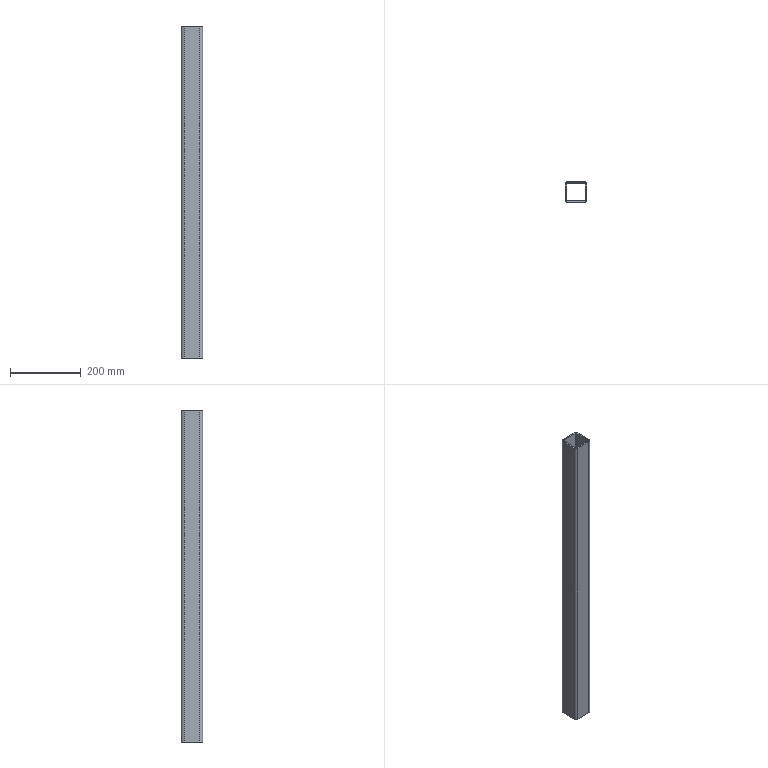Part | SolidWorks | features ICE 1, LibraryFeature 1 | 1 solid | 18 faces | box 60 x 60 x 940 mm | volume 803509 mm3 | plane 10 | cylinder 8 | commonest cylinder face diameters 8 x4 16 x4
STEP:
#1=CARTESIAN_POINT('',(22.,30.,0.));
#2=VERTEX_POINT('',#1);
#3=CARTESIAN_POINT('',(-22.,30.,0.));
#4=VERTEX_POINT('',#3);
#5=CARTESIAN_POINT('',(0.,30.,0.));
#6=DIRECTION('',(-1.,0.,0.));
#7=VECTOR('',#6,1000.);
#8=LINE('',#5,#7);
#9=EDGE_CURVE('',#2,#4,#8,.T.);
#10=ORIENTED_EDGE('',*,*,#9,.T.);
#11=CARTESIAN_POINT('',(-22.,30.,940.));
#12=VERTEX_POINT('',#11);
#13=CARTESIAN_POINT('',(-22.,30.,940.));
#14=DIRECTION('',(0.,0.,-1.));
#15=VECTOR('',#14,1000.);
#16=LINE('',#13,#15);
#17=EDGE_CURVE('',#12,#4,#16,.T.);
#18=ORIENTED_EDGE('',*,*,#17,.F.);
#19=CARTESIAN_POINT('',(22.,30.,940.));
#20=VERTEX_POINT('',#19);
#21=CARTESIAN_POINT('',(0.,30.,940.));
#22=DIRECTION('',(-1.,0.,0.));
#23=VECTOR('',#22,1000.);
#24=LINE('',#21,#23);
#25=EDGE_CURVE('',#20,#12,#24,.T.);
#26=ORIENTED_EDGE('',*,*,#25,.F.);
#27=CARTESIAN_POINT('',(22.,30.,940.));
#28=DIRECTION('',(0.,0.,-1.));
#29=VECTOR('',#28,1000.);
#30=LINE('',#27,#29);
#31=EDGE_CURVE('',#20,#2,#30,.T.);
#32=ORIENTED_EDGE('',*,*,#31,.T.);
#33=EDGE_LOOP('',(#10,#18,#26,#32));
#34=FACE_OUTER_BOUND('',#33,.T.);
#35=CARTESIAN_POINT('',(0.,30.,940.));
#36=DIRECTION('',(0.,-1.,0.));
#37=DIRECTION('',(0.,0.,-1.));
#38=AXIS2_PLACEMENT_3D('',#35,#36,#37);
#39=PLANE('',#38);
#40=ADVANCED_FACE('',(#34),#39,.F.);
#41=CARTESIAN_POINT('',(-30.,22.,0.));
#42=VERTEX_POINT('',#41);
#43=CARTESIAN_POINT('',(-22.,22.,0.));
#44=DIRECTION('',(0.,0.,1.));
#45=DIRECTION('',(1.,0.,0.));
#46=AXIS2_PLACEMENT_3D('',#43,#44,#45);
#47=CIRCLE('',#46,8.);
#48=EDGE_CURVE('',#4,#42,#47,.T.);
#49=ORIENTED_EDGE('',*,*,#48,.T.);
#50=CARTESIAN_POINT('',(-30.,22.,940.));
#51=VERTEX_POINT('',#50);
#52=CARTESIAN_POINT('',(-30.,22.,940.));
#53=DIRECTION('',(0.,0.,-1.));
#54=VECTOR('',#53,1000.);
#55=LINE('',#52,#54);
#56=EDGE_CURVE('',#51,#42,#55,.T.);
#57=ORIENTED_EDGE('',*,*,#56,.F.);
#58=CARTESIAN_POINT('',(-22.,22.,940.));
#59=DIRECTION('',(0.,0.,1.));
#60=DIRECTION('',(1.,0.,0.));
#61=AXIS2_PLACEMENT_3D('',#58,#59,#60);
#62=CIRCLE('',#61,8.);
#63=EDGE_CURVE('',#12,#51,#62,.T.);
#64=ORIENTED_EDGE('',*,*,#63,.F.);
#65=ORIENTED_EDGE('',*,*,#17,.T.);
#66=EDGE_LOOP('',(#49,#57,#64,#65));
#67=FACE_OUTER_BOUND('',#66,.T.);
#68=CARTESIAN_POINT('',(-22.,22.,940.));
#69=DIRECTION('',(0.,0.,-1.));
#70=DIRECTION('',(-1.,0.,0.));
#71=AXIS2_PLACEMENT_3D('',#68,#69,#70);
#72=CYLINDRICAL_SURFACE('',#71,8.);
#73=ADVANCED_FACE('',(#67),#72,.T.);
#74=CARTESIAN_POINT('',(-30.,-22.,0.));
#75=VERTEX_POINT('',#74);
#76=CARTESIAN_POINT('',(-30.,0.,0.));
#77=DIRECTION('',(0.,1.,0.));
#78=VECTOR('',#77,1000.);
#79=LINE('',#76,#78);
#80=EDGE_CURVE('',#75,#42,#79,.T.);
#81=ORIENTED_EDGE('',*,*,#80,.F.);
#82=CARTESIAN_POINT('',(-30.,-22.,940.));
#83=VERTEX_POINT('',#82);
#84=CARTESIAN_POINT('',(-30.,-22.,940.));
#85=DIRECTION('',(0.,0.,-1.));
#86=VECTOR('',#85,1000.);
#87=LINE('',#84,#86);
#88=EDGE_CURVE('',#83,#75,#87,.T.);
#89=ORIENTED_EDGE('',*,*,#88,.F.);
#90=CARTESIAN_POINT('',(-30.,0.,940.));
#91=DIRECTION('',(0.,1.,0.));
#92=VECTOR('',#91,1000.);
#93=LINE('',#90,#92);
#94=EDGE_CURVE('',#83,#51,#93,.T.);
#95=ORIENTED_EDGE('',*,*,#94,.T.);
#96=ORIENTED_EDGE('',*,*,#56,.T.);
#97=EDGE_LOOP('',(#81,#89,#95,#96));
#98=FACE_OUTER_BOUND('',#97,.T.);
#99=CARTESIAN_POINT('',(-30.,0.,940.));
#100=DIRECTION('',(-1.,0.,0.));
#101=DIRECTION('',(0.,0.,1.));
#102=AXIS2_PLACEMENT_3D('',#99,#100,#101);
#103=PLANE('',#102);
#104=ADVANCED_FACE('',(#98),#103,.T.);
#105=CARTESIAN_POINT('',(-22.,-30.,0.));
#106=VERTEX_POINT('',#105);
#107=CARTESIAN_POINT('',(-22.,-22.,0.));
#108=DIRECTION('',(0.,0.,1.));
#109=DIRECTION('',(1.,0.,0.));
#110=AXIS2_PLACEMENT_3D('',#107,#108,#109);
#111=CIRCLE('',#110,8.);
#112=EDGE_CURVE('',#75,#106,#111,.T.);
#113=ORIENTED_EDGE('',*,*,#112,.T.);
#114=CARTESIAN_POINT('',(-22.,-30.,940.));
#115=VERTEX_POINT('',#114);
#116=CARTESIAN_POINT('',(-22.,-30.,940.));
#117=DIRECTION('',(0.,0.,-1.));
#118=VECTOR('',#117,1000.);
#119=LINE('',#116,#118);
#120=EDGE_CURVE('',#115,#106,#119,.T.);
#121=ORIENTED_EDGE('',*,*,#120,.F.);
#122=CARTESIAN_POINT('',(-22.,-22.,940.));
#123=DIRECTION('',(0.,0.,1.));
#124=DIRECTION('',(1.,0.,0.));
#125=AXIS2_PLACEMENT_3D('',#122,#123,#124);
#126=CIRCLE('',#125,8.);
#127=EDGE_CURVE('',#83,#115,#126,.T.);
#128=ORIENTED_EDGE('',*,*,#127,.F.);
#129=ORIENTED_EDGE('',*,*,#88,.T.);
#130=EDGE_LOOP('',(#113,#121,#128,#129));
#131=FACE_OUTER_BOUND('',#130,.T.);
#132=CARTESIAN_POINT('',(-22.,-22.,940.));
#133=DIRECTION('',(0.,0.,-1.));
#134=DIRECTION('',(-1.,0.,0.));
#135=AXIS2_PLACEMENT_3D('',#132,#133,#134);
#136=CYLINDRICAL_SURFACE('',#135,8.);
#137=ADVANCED_FACE('',(#131),#136,.T.);
#138=CARTESIAN_POINT('',(22.,-30.,0.));
#139=VERTEX_POINT('',#138);
#140=CARTESIAN_POINT('',(0.,-30.,0.));
#141=DIRECTION('',(1.,0.,0.));
#142=VECTOR('',#141,1000.);
#143=LINE('',#140,#142);
#144=EDGE_CURVE('',#106,#139,#143,.T.);
#145=ORIENTED_EDGE('',*,*,#144,.T.);
#146=CARTESIAN_POINT('',(22.,-30.,940.));
#147=VERTEX_POINT('',#146);
#148=CARTESIAN_POINT('',(22.,-30.,940.));
#149=DIRECTION('',(0.,0.,-1.));
#150=VECTOR('',#149,1000.);
#151=LINE('',#148,#150);
#152=EDGE_CURVE('',#147,#139,#151,.T.);
#153=ORIENTED_EDGE('',*,*,#152,.F.);
#154=CARTESIAN_POINT('',(0.,-30.,940.));
#155=DIRECTION('',(1.,0.,0.));
#156=VECTOR('',#155,1000.);
#157=LINE('',#154,#156);
#158=EDGE_CURVE('',#115,#147,#157,.T.);
#159=ORIENTED_EDGE('',*,*,#158,.F.);
#160=ORIENTED_EDGE('',*,*,#120,.T.);
#161=EDGE_LOOP('',(#145,#153,#159,#160));
#162=FACE_OUTER_BOUND('',#161,.T.);
#163=CARTESIAN_POINT('',(0.,-30.,940.));
#164=DIRECTION('',(0.,1.,0.));
#165=DIRECTION('',(0.,0.,1.));
#166=AXIS2_PLACEMENT_3D('',#163,#164,#165);
#167=PLANE('',#166);
#168=ADVANCED_FACE('',(#162),#167,.F.);
#169=CARTESIAN_POINT('',(30.,-22.,0.));
#170=VERTEX_POINT('',#169);
#171=CARTESIAN_POINT('',(22.,-22.,0.));
#172=DIRECTION('',(0.,0.,1.));
#173=DIRECTION('',(1.,0.,0.));
#174=AXIS2_PLACEMENT_3D('',#171,#172,#173);
#175=CIRCLE('',#174,8.);
#176=EDGE_CURVE('',#139,#170,#175,.T.);
#177=ORIENTED_EDGE('',*,*,#176,.T.);
#178=CARTESIAN_POINT('',(30.,-22.,940.));
#179=VERTEX_POINT('',#178);
#180=CARTESIAN_POINT('',(30.,-22.,940.));
#181=DIRECTION('',(0.,0.,-1.));
#182=VECTOR('',#181,1000.);
#183=LINE('',#180,#182);
#184=EDGE_CURVE('',#179,#170,#183,.T.);
#185=ORIENTED_EDGE('',*,*,#184,.F.);
#186=CARTESIAN_POINT('',(22.,-22.,940.));
#187=DIRECTION('',(0.,0.,1.));
#188=DIRECTION('',(1.,0.,0.));
#189=AXIS2_PLACEMENT_3D('',#186,#187,#188);
#190=CIRCLE('',#189,8.);
#191=EDGE_CURVE('',#147,#179,#190,.T.);
#192=ORIENTED_EDGE('',*,*,#191,.F.);
#193=ORIENTED_EDGE('',*,*,#152,.T.);
#194=EDGE_LOOP('',(#177,#185,#192,#193));
#195=FACE_OUTER_BOUND('',#194,.T.);
#196=CARTESIAN_POINT('',(22.,-22.,940.));
#197=DIRECTION('',(0.,0.,-1.));
#198=DIRECTION('',(-1.,0.,0.));
#199=AXIS2_PLACEMENT_3D('',#196,#197,#198);
#200=CYLINDRICAL_SURFACE('',#199,8.);
#201=ADVANCED_FACE('',(#195),#200,.T.);
#202=CARTESIAN_POINT('',(30.,22.,0.));
#203=VERTEX_POINT('',#202);
#204=CARTESIAN_POINT('',(30.,0.,0.));
#205=DIRECTION('',(0.,-1.,0.));
#206=VECTOR('',#205,1000.);
#207=LINE('',#204,#206);
#208=EDGE_CURVE('',#203,#170,#207,.T.);
#209=ORIENTED_EDGE('',*,*,#208,.F.);
#210=CARTESIAN_POINT('',(30.,22.,940.));
#211=VERTEX_POINT('',#210);
#212=CARTESIAN_POINT('',(30.,22.,940.));
#213=DIRECTION('',(0.,0.,-1.));
#214=VECTOR('',#213,1000.);
#215=LINE('',#212,#214);
#216=EDGE_CURVE('',#211,#203,#215,.T.);
#217=ORIENTED_EDGE('',*,*,#216,.F.);
#218=CARTESIAN_POINT('',(30.,0.,940.));
#219=DIRECTION('',(0.,-1.,0.));
#220=VECTOR('',#219,1000.);
#221=LINE('',#218,#220);
#222=EDGE_CURVE('',#211,#179,#221,.T.);
#223=ORIENTED_EDGE('',*,*,#222,.T.);
#224=ORIENTED_EDGE('',*,*,#184,.T.);
#225=EDGE_LOOP('',(#209,#217,#223,#224));
#226=FACE_OUTER_BOUND('',#225,.T.);
#227=CARTESIAN_POINT('',(30.,0.,940.));
#228=DIRECTION('',(1.,0.,0.));
#229=DIRECTION('',(0.,0.,-1.));
#230=AXIS2_PLACEMENT_3D('',#227,#228,#229);
#231=PLANE('',#230);
#232=ADVANCED_FACE('',(#226),#231,.T.);
#233=CARTESIAN_POINT('',(-26.,-22.,0.));
#234=VERTEX_POINT('',#233);
#235=CARTESIAN_POINT('',(-22.,-26.,0.));
#236=VERTEX_POINT('',#235);
#237=CARTESIAN_POINT('',(-22.,-22.,0.));
#238=DIRECTION('',(0.,0.,1.));
#239=DIRECTION('',(1.,0.,0.));
#240=AXIS2_PLACEMENT_3D('',#237,#238,#239);
#241=CIRCLE('',#240,4.);
#242=EDGE_CURVE('',#234,#236,#241,.T.);
#243=ORIENTED_EDGE('',*,*,#242,.F.);
#244=CARTESIAN_POINT('',(-26.,-22.,940.));
#245=VERTEX_POINT('',#244);
#246=CARTESIAN_POINT('',(-26.,-22.,940.));
#247=DIRECTION('',(0.,0.,-1.));
#248=VECTOR('',#247,1000.);
#249=LINE('',#246,#248);
#250=EDGE_CURVE('',#245,#234,#249,.T.);
#251=ORIENTED_EDGE('',*,*,#250,.F.);
#252=CARTESIAN_POINT('',(-22.,-26.,940.));
#253=VERTEX_POINT('',#252);
#254=CARTESIAN_POINT('',(-22.,-22.,940.));
#255=DIRECTION('',(0.,0.,1.));
#256=DIRECTION('',(1.,0.,0.));
#257=AXIS2_PLACEMENT_3D('',#254,#255,#256);
#258=CIRCLE('',#257,4.);
#259=EDGE_CURVE('',#245,#253,#258,.T.);
#260=ORIENTED_EDGE('',*,*,#259,.T.);
#261=CARTESIAN_POINT('',(-22.,-26.,940.));
#262=DIRECTION('',(0.,0.,-1.));
#263=VECTOR('',#262,1000.);
#264=LINE('',#261,#263);
#265=EDGE_CURVE('',#253,#236,#264,.T.);
#266=ORIENTED_EDGE('',*,*,#265,.T.);
#267=EDGE_LOOP('',(#243,#251,#260,#266));
#268=FACE_OUTER_BOUND('',#267,.T.);
#269=CARTESIAN_POINT('',(-22.,-22.,940.));
#270=DIRECTION('',(0.,0.,-1.));
#271=DIRECTION('',(-1.,0.,0.));
#272=AXIS2_PLACEMENT_3D('',#269,#270,#271);
#273=CYLINDRICAL_SURFACE('',#272,4.);
#274=ADVANCED_FACE('',(#268),#273,.F.);
#275=CARTESIAN_POINT('',(-26.,22.,0.));
#276=VERTEX_POINT('',#275);
#277=CARTESIAN_POINT('',(-26.,0.,0.));
#278=DIRECTION('',(0.,1.,0.));
#279=VECTOR('',#278,1000.);
#280=LINE('',#277,#279);
#281=EDGE_CURVE('',#234,#276,#280,.T.);
#282=ORIENTED_EDGE('',*,*,#281,.T.);
#283=CARTESIAN_POINT('',(-26.,22.,940.));
#284=VERTEX_POINT('',#283);
#285=CARTESIAN_POINT('',(-26.,22.,940.));
#286=DIRECTION('',(0.,0.,-1.));
#287=VECTOR('',#286,1000.);
#288=LINE('',#285,#287);
#289=EDGE_CURVE('',#284,#276,#288,.T.);
#290=ORIENTED_EDGE('',*,*,#289,.F.);
#291=CARTESIAN_POINT('',(-26.,0.,940.));
#292=DIRECTION('',(0.,1.,0.));
#293=VECTOR('',#292,1000.);
#294=LINE('',#291,#293);
#295=EDGE_CURVE('',#245,#284,#294,.T.);
#296=ORIENTED_EDGE('',*,*,#295,.F.);
#297=ORIENTED_EDGE('',*,*,#250,.T.);
#298=EDGE_LOOP('',(#282,#290,#296,#297));
#299=FACE_OUTER_BOUND('',#298,.T.);
#300=CARTESIAN_POINT('',(-26.,0.,940.));
#301=DIRECTION('',(-1.,0.,0.));
#302=DIRECTION('',(0.,0.,1.));
#303=AXIS2_PLACEMENT_3D('',#300,#301,#302);
#304=PLANE('',#303);
#305=ADVANCED_FACE('',(#299),#304,.F.);
#306=CARTESIAN_POINT('',(-22.,26.,0.));
#307=VERTEX_POINT('',#306);
#308=CARTESIAN_POINT('',(-22.,22.,0.));
#309=DIRECTION('',(0.,0.,1.));
#310=DIRECTION('',(1.,0.,0.));
#311=AXIS2_PLACEMENT_3D('',#308,#309,#310);
#312=CIRCLE('',#311,4.);
#313=EDGE_CURVE('',#307,#276,#312,.T.);
#314=ORIENTED_EDGE('',*,*,#313,.F.);
#315=CARTESIAN_POINT('',(-22.,26.,940.));
#316=VERTEX_POINT('',#315);
#317=CARTESIAN_POINT('',(-22.,26.,940.));
#318=DIRECTION('',(0.,0.,-1.));
#319=VECTOR('',#318,1000.);
#320=LINE('',#317,#319);
#321=EDGE_CURVE('',#316,#307,#320,.T.);
#322=ORIENTED_EDGE('',*,*,#321,.F.);
#323=CARTESIAN_POINT('',(-22.,22.,940.));
#324=DIRECTION('',(0.,0.,1.));
#325=DIRECTION('',(1.,0.,0.));
#326=AXIS2_PLACEMENT_3D('',#323,#324,#325);
#327=CIRCLE('',#326,4.);
#328=EDGE_CURVE('',#316,#284,#327,.T.);
#329=ORIENTED_EDGE('',*,*,#328,.T.);
#330=ORIENTED_EDGE('',*,*,#289,.T.);
#331=EDGE_LOOP('',(#314,#322,#329,#330));
#332=FACE_OUTER_BOUND('',#331,.T.);
#333=CARTESIAN_POINT('',(-22.,22.,940.));
#334=DIRECTION('',(0.,0.,-1.));
#335=DIRECTION('',(-1.,0.,0.));
#336=AXIS2_PLACEMENT_3D('',#333,#334,#335);
#337=CYLINDRICAL_SURFACE('',#336,4.);
#338=ADVANCED_FACE('',(#332),#337,.F.);
#339=CARTESIAN_POINT('',(22.,26.,0.));
#340=VERTEX_POINT('',#339);
#341=CARTESIAN_POINT('',(0.,26.,0.));
#342=DIRECTION('',(-1.,0.,0.));
#343=VECTOR('',#342,1000.);
#344=LINE('',#341,#343);
#345=EDGE_CURVE('',#340,#307,#344,.T.);
#346=ORIENTED_EDGE('',*,*,#345,.F.);
#347=CARTESIAN_POINT('',(22.,26.,940.));
#348=VERTEX_POINT('',#347);
#349=CARTESIAN_POINT('',(22.,26.,940.));
#350=DIRECTION('',(0.,0.,-1.));
#351=VECTOR('',#350,1000.);
#352=LINE('',#349,#351);
#353=EDGE_CURVE('',#348,#340,#352,.T.);
#354=ORIENTED_EDGE('',*,*,#353,.F.);
#355=CARTESIAN_POINT('',(0.,26.,940.));
#356=DIRECTION('',(-1.,0.,0.));
#357=VECTOR('',#356,1000.);
#358=LINE('',#355,#357);
#359=EDGE_CURVE('',#348,#316,#358,.T.);
#360=ORIENTED_EDGE('',*,*,#359,.T.);
#361=ORIENTED_EDGE('',*,*,#321,.T.);
#362=EDGE_LOOP('',(#346,#354,#360,#361));
#363=FACE_OUTER_BOUND('',#362,.T.);
#364=CARTESIAN_POINT('',(0.,26.,940.));
#365=DIRECTION('',(0.,-1.,0.));
#366=DIRECTION('',(0.,0.,-1.));
#367=AXIS2_PLACEMENT_3D('',#364,#365,#366);
#368=PLANE('',#367);
#369=ADVANCED_FACE('',(#363),#368,.T.);
#370=CARTESIAN_POINT('',(26.,22.,0.));
#371=VERTEX_POINT('',#370);
#372=CARTESIAN_POINT('',(22.,22.,0.));
#373=DIRECTION('',(0.,0.,1.));
#374=DIRECTION('',(1.,0.,0.));
#375=AXIS2_PLACEMENT_3D('',#372,#373,#374);
#376=CIRCLE('',#375,4.);
#377=EDGE_CURVE('',#371,#340,#376,.T.);
#378=ORIENTED_EDGE('',*,*,#377,.F.);
#379=CARTESIAN_POINT('',(26.,22.,940.));
#380=VERTEX_POINT('',#379);
#381=CARTESIAN_POINT('',(26.,22.,940.));
#382=DIRECTION('',(0.,0.,-1.));
#383=VECTOR('',#382,1000.);
#384=LINE('',#381,#383);
#385=EDGE_CURVE('',#380,#371,#384,.T.);
#386=ORIENTED_EDGE('',*,*,#385,.F.);
#387=CARTESIAN_POINT('',(22.,22.,940.));
#388=DIRECTION('',(0.,0.,1.));
#389=DIRECTION('',(1.,0.,0.));
#390=AXIS2_PLACEMENT_3D('',#387,#388,#389);
#391=CIRCLE('',#390,4.);
#392=EDGE_CURVE('',#380,#348,#391,.T.);
#393=ORIENTED_EDGE('',*,*,#392,.T.);
#394=ORIENTED_EDGE('',*,*,#353,.T.);
#395=EDGE_LOOP('',(#378,#386,#393,#394));
#396=FACE_OUTER_BOUND('',#395,.T.);
#397=CARTESIAN_POINT('',(22.,22.,940.));
#398=DIRECTION('',(0.,0.,-1.));
#399=DIRECTION('',(-1.,0.,0.));
#400=AXIS2_PLACEMENT_3D('',#397,#398,#399);
#401=CYLINDRICAL_SURFACE('',#400,4.);
#402=ADVANCED_FACE('',(#396),#401,.F.);
#403=CARTESIAN_POINT('',(26.,-22.,0.));
#404=VERTEX_POINT('',#403);
#405=CARTESIAN_POINT('',(26.,0.,0.));
#406=DIRECTION('',(0.,-1.,0.));
#407=VECTOR('',#406,1000.);
#408=LINE('',#405,#407);
#409=EDGE_CURVE('',#371,#404,#408,.T.);
#410=ORIENTED_EDGE('',*,*,#409,.T.);
#411=CARTESIAN_POINT('',(26.,-22.,940.));
#412=VERTEX_POINT('',#411);
#413=CARTESIAN_POINT('',(26.,-22.,940.));
#414=DIRECTION('',(0.,0.,-1.));
#415=VECTOR('',#414,1000.);
#416=LINE('',#413,#415);
#417=EDGE_CURVE('',#412,#404,#416,.T.);
#418=ORIENTED_EDGE('',*,*,#417,.F.);
#419=CARTESIAN_POINT('',(26.,0.,940.));
#420=DIRECTION('',(0.,-1.,0.));
#421=VECTOR('',#420,1000.);
#422=LINE('',#419,#421);
#423=EDGE_CURVE('',#380,#412,#422,.T.);
#424=ORIENTED_EDGE('',*,*,#423,.F.);
#425=ORIENTED_EDGE('',*,*,#385,.T.);
#426=EDGE_LOOP('',(#410,#418,#424,#425));
#427=FACE_OUTER_BOUND('',#426,.T.);
#428=CARTESIAN_POINT('',(26.,0.,940.));
#429=DIRECTION('',(1.,0.,0.));
#430=DIRECTION('',(0.,0.,-1.));
#431=AXIS2_PLACEMENT_3D('',#428,#429,#430);
#432=PLANE('',#431);
#433=ADVANCED_FACE('',(#427),#432,.F.);
#434=CARTESIAN_POINT('',(22.,-26.,0.));
#435=VERTEX_POINT('',#434);
#436=CARTESIAN_POINT('',(22.,-22.,0.));
#437=DIRECTION('',(0.,0.,1.));
#438=DIRECTION('',(1.,0.,0.));
#439=AXIS2_PLACEMENT_3D('',#436,#437,#438);
#440=CIRCLE('',#439,4.);
#441=EDGE_CURVE('',#435,#404,#440,.T.);
#442=ORIENTED_EDGE('',*,*,#441,.F.);
#443=CARTESIAN_POINT('',(22.,-26.,940.));
#444=VERTEX_POINT('',#443);
#445=CARTESIAN_POINT('',(22.,-26.,940.));
#446=DIRECTION('',(0.,0.,-1.));
#447=VECTOR('',#446,1000.);
#448=LINE('',#445,#447);
#449=EDGE_CURVE('',#444,#435,#448,.T.);
#450=ORIENTED_EDGE('',*,*,#449,.F.);
#451=CARTESIAN_POINT('',(22.,-22.,940.));
#452=DIRECTION('',(0.,0.,1.));
#453=DIRECTION('',(1.,0.,0.));
#454=AXIS2_PLACEMENT_3D('',#451,#452,#453);
#455=CIRCLE('',#454,4.);
#456=EDGE_CURVE('',#444,#412,#455,.T.);
#457=ORIENTED_EDGE('',*,*,#456,.T.);
#458=ORIENTED_EDGE('',*,*,#417,.T.);
#459=EDGE_LOOP('',(#442,#450,#457,#458));
#460=FACE_OUTER_BOUND('',#459,.T.);
#461=CARTESIAN_POINT('',(22.,-22.,940.));
#462=DIRECTION('',(0.,0.,-1.));
#463=DIRECTION('',(-1.,0.,0.));
#464=AXIS2_PLACEMENT_3D('',#461,#462,#463);
#465=CYLINDRICAL_SURFACE('',#464,4.);
#466=ADVANCED_FACE('',(#460),#465,.F.);
#467=CARTESIAN_POINT('',(0.,-26.,0.));
#468=DIRECTION('',(1.,0.,0.));
#469=VECTOR('',#468,1000.);
#470=LINE('',#467,#469);
#471=EDGE_CURVE('',#236,#435,#470,.T.);
#472=ORIENTED_EDGE('',*,*,#471,.F.);
#473=ORIENTED_EDGE('',*,*,#265,.F.);
#474=CARTESIAN_POINT('',(0.,-26.,940.));
#475=DIRECTION('',(1.,0.,0.));
#476=VECTOR('',#475,1000.);
#477=LINE('',#474,#476);
#478=EDGE_CURVE('',#253,#444,#477,.T.);
#479=ORIENTED_EDGE('',*,*,#478,.T.);
#480=ORIENTED_EDGE('',*,*,#449,.T.);
#481=EDGE_LOOP('',(#472,#473,#479,#480));
#482=FACE_OUTER_BOUND('',#481,.T.);
#483=CARTESIAN_POINT('',(0.,-26.,940.));
#484=DIRECTION('',(0.,1.,0.));
#485=DIRECTION('',(0.,0.,1.));
#486=AXIS2_PLACEMENT_3D('',#483,#484,#485);
#487=PLANE('',#486);
#488=ADVANCED_FACE('',(#482),#487,.T.);
#489=CARTESIAN_POINT('',(22.,22.,0.));
#490=DIRECTION('',(0.,0.,1.));
#491=DIRECTION('',(1.,0.,0.));
#492=AXIS2_PLACEMENT_3D('',#489,#490,#491);
#493=CIRCLE('',#492,8.);
#494=EDGE_CURVE('',#203,#2,#493,.T.);
#495=ORIENTED_EDGE('',*,*,#494,.T.);
#496=ORIENTED_EDGE('',*,*,#31,.F.);
#497=CARTESIAN_POINT('',(22.,22.,940.));
#498=DIRECTION('',(0.,0.,1.));
#499=DIRECTION('',(1.,0.,0.));
#500=AXIS2_PLACEMENT_3D('',#497,#498,#499);
#501=CIRCLE('',#500,8.);
#502=EDGE_CURVE('',#211,#20,#501,.T.);
#503=ORIENTED_EDGE('',*,*,#502,.F.);
#504=ORIENTED_EDGE('',*,*,#216,.T.);
#505=EDGE_LOOP('',(#495,#496,#503,#504));
#506=FACE_OUTER_BOUND('',#505,.T.);
#507=CARTESIAN_POINT('',(22.,22.,940.));
#508=DIRECTION('',(0.,0.,-1.));
#509=DIRECTION('',(-1.,0.,0.));
#510=AXIS2_PLACEMENT_3D('',#507,#508,#509);
#511=CYLINDRICAL_SURFACE('',#510,8.);
#512=ADVANCED_FACE('',(#506),#511,.T.);
#513=ORIENTED_EDGE('',*,*,#259,.F.);
#514=ORIENTED_EDGE('',*,*,#295,.T.);
#515=ORIENTED_EDGE('',*,*,#328,.F.);
#516=ORIENTED_EDGE('',*,*,#359,.F.);
#517=ORIENTED_EDGE('',*,*,#392,.F.);
#518=ORIENTED_EDGE('',*,*,#423,.T.);
#519=ORIENTED_EDGE('',*,*,#456,.F.);
#520=ORIENTED_EDGE('',*,*,#478,.F.);
#521=EDGE_LOOP('',(#513,#514,#515,#516,#517,#518,#519,#520));
#522=FACE_BOUND('',#521,.T.);
#523=ORIENTED_EDGE('',*,*,#25,.T.);
#524=ORIENTED_EDGE('',*,*,#63,.T.);
#525=ORIENTED_EDGE('',*,*,#94,.F.);
#526=ORIENTED_EDGE('',*,*,#127,.T.);
#527=ORIENTED_EDGE('',*,*,#158,.T.);
#528=ORIENTED_EDGE('',*,*,#191,.T.);
#529=ORIENTED_EDGE('',*,*,#222,.F.);
#530=ORIENTED_EDGE('',*,*,#502,.T.);
#531=EDGE_LOOP('',(#523,#524,#525,#526,#527,#528,#529,#530));
#532=FACE_OUTER_BOUND('',#531,.T.);
#533=CARTESIAN_POINT('',(0.,0.,940.));
#534=DIRECTION('',(0.,0.,1.));
#535=DIRECTION('',(1.,0.,0.));
#536=AXIS2_PLACEMENT_3D('',#533,#534,#535);
#537=PLANE('',#536);
#538=ADVANCED_FACE('',(#522,#532),#537,.T.);
#539=ORIENTED_EDGE('',*,*,#242,.T.);
#540=ORIENTED_EDGE('',*,*,#471,.T.);
#541=ORIENTED_EDGE('',*,*,#441,.T.);
#542=ORIENTED_EDGE('',*,*,#409,.F.);
#543=ORIENTED_EDGE('',*,*,#377,.T.);
#544=ORIENTED_EDGE('',*,*,#345,.T.);
#545=ORIENTED_EDGE('',*,*,#313,.T.);
#546=ORIENTED_EDGE('',*,*,#281,.F.);
#547=EDGE_LOOP('',(#539,#540,#541,#542,#543,#544,#545,#546));
#548=FACE_BOUND('',#547,.T.);
#549=ORIENTED_EDGE('',*,*,#9,.F.);
#550=ORIENTED_EDGE('',*,*,#494,.F.);
#551=ORIENTED_EDGE('',*,*,#208,.T.);
#552=ORIENTED_EDGE('',*,*,#176,.F.);
#553=ORIENTED_EDGE('',*,*,#144,.F.);
#554=ORIENTED_EDGE('',*,*,#112,.F.);
#555=ORIENTED_EDGE('',*,*,#80,.T.);
#556=ORIENTED_EDGE('',*,*,#48,.F.);
#557=EDGE_LOOP('',(#549,#550,#551,#552,#553,#554,#555,#556));
#558=FACE_OUTER_BOUND('',#557,.T.);
#559=CARTESIAN_POINT('',(0.,0.,0.));
#560=DIRECTION('',(0.,0.,1.));
#561=DIRECTION('',(1.,0.,0.));
#562=AXIS2_PLACEMENT_3D('',#559,#560,#561);
#563=PLANE('',#562);
#564=ADVANCED_FACE('',(#548,#558),#563,.F.);
#565=CLOSED_SHELL('',(#40,#73,#104,#137,#168,#201,#232,#274,#305,#338,#369,#402,#433,#466,#488,#512,#538,#564));
#566=MANIFOLD_SOLID_BREP('',#565);
#567=CARTESIAN_POINT('',(0.,0.,0.));
#568=DIRECTION('',(0.,0.,1.));
#569=DIRECTION('',(1.,0.,0.));
#570=AXIS2_PLACEMENT_3D('',#567,#568,#569);
#571=(LENGTH_UNIT()NAMED_UNIT(*)SI_UNIT(.MILLI.,.METRE.));
#572=UNCERTAINTY_MEASURE_WITH_UNIT(LENGTH_MEASURE(0.00001),#571,'','');
#573=(NAMED_UNIT(*)PLANE_ANGLE_UNIT()SI_UNIT($,.RADIAN.));
#574=(NAMED_UNIT(*)SI_UNIT($,.STERADIAN.)SOLID_ANGLE_UNIT());
#575=(GEOMETRIC_REPRESENTATION_CONTEXT(3)GLOBAL_UNCERTAINTY_ASSIGNED_CONTEXT((#572))GLOBAL_UNIT_ASSIGNED_CONTEXT((#571,#573,#574))REPRESENTATION_CONTEXT('',''));
#576=ADVANCED_BREP_SHAPE_REPRESENTATION('',(#566,#570),#575);